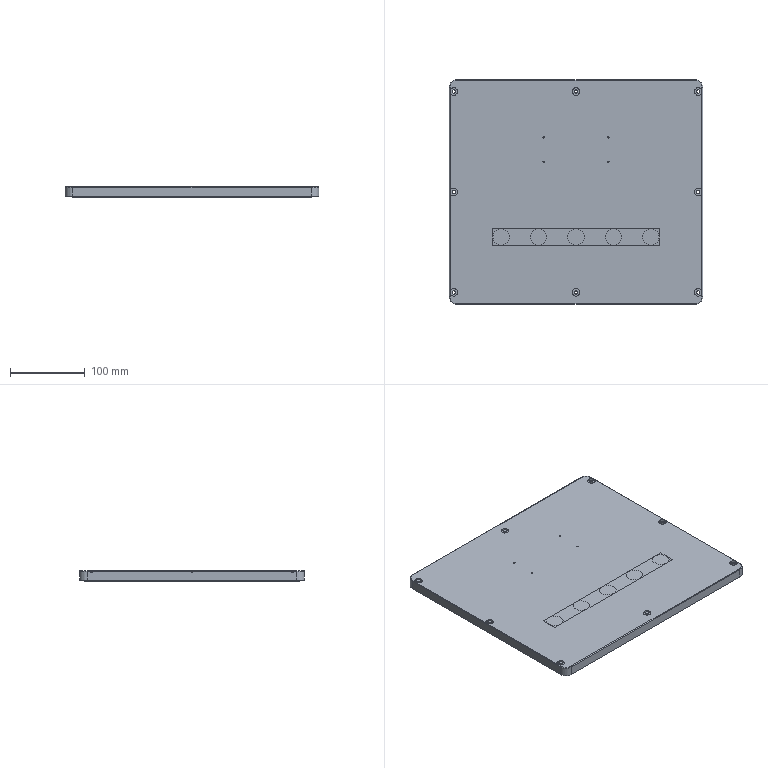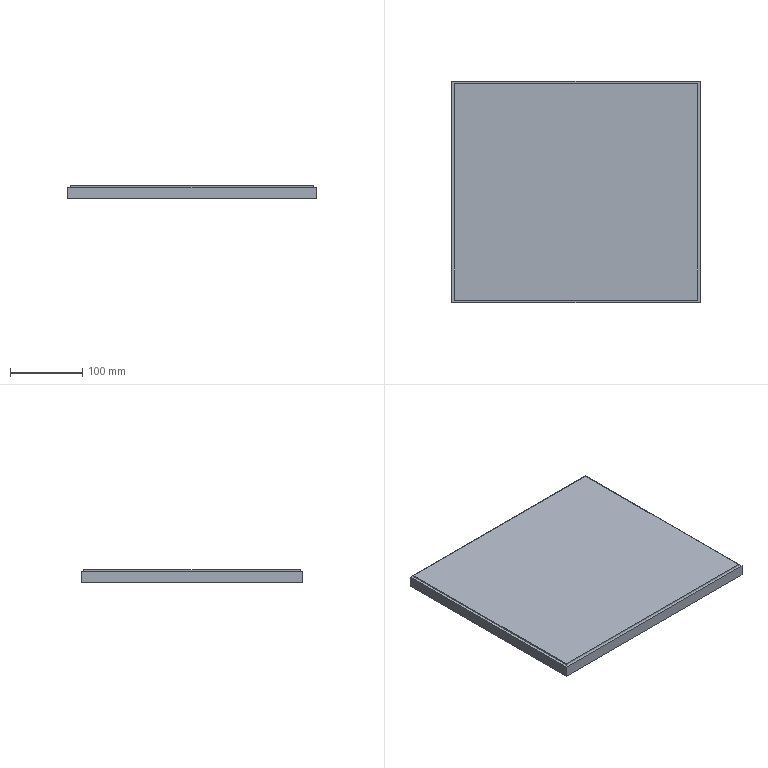CAM job | NX | 3-axis milling, drilling | part box 338 x 300 x 14.5 mm | stock box 345 x 307 x 18 mm
Tools:
number,name,description,diameter,corner_radius,flute_length,length,flutes
3,D63,Milling Tool-5 Parameters,63.0,0.0,50.0,75.0,2
4,D10,Milling Tool-5 Parameters,10.0,0.0,50.0,75.0,2
14,D10JING,Milling Tool-5 Parameters,10.0,0.0,50.0,75.0,2
1,D6A45,Milling Tool-5 Parameters,6.0,0.0,3.0,3.0,2
20,2.1ZT,Drilling Tool,2.05,0.0,35.0,50.0,2
11,4.5ZT,Drilling Tool,4.5,0.0,35.0,50.0,2
7,D3R0.5,Milling Tool-5 Parameters,3.0,0.5,50.0,75.0,2
16,D6,Milling Tool-5 Parameters,6.0,0.0,50.0,75.0,2
22,2.5ZT,Drilling Tool,2.5,0.0,35.0,50.0,2
21,D4A45,Milling Tool-5 Parameters,4.0,0.0,2.0,2.0,2
17,D4,Milling Tool-5 Parameters,4.0,0.0,50.0,75.0,2
Operations:
program,operation,operation_type,tool,method,geometry_group,spindle_rpm,surface_speed,feed_per_tooth,feed_cut,feed_plunge,cut_length_mm,path_length_mm,cut_time_min,machine_time_min
1,FLOOR_WALL,VolumeBased25DMillingOperation,D63,METHOD,A,6500.0,1286.0,0.0962,1250.0,100.0,3149.797,3203.797,2.52,2.525
1,DRILLING_COPY_1,Operation,D6A45,METHOD,A,5000.0,94.0,0.025,250.0,0.0,61.2,1674.06,0.2448,0.4061
1,DRILLING_COPY_COPY,Operation,2.1ZT,METHOD,A,1447.0,10.0,0.0346,100.0,0.0,40.464,302.252,0.4046,0.4308
1,DRILLING_COPY_COPY_COPY,Operation,4.5ZT,METHOD,A,1447.0,10.0,0.0346,100.0,0.0,146.815,1399.848,1.468,1.593
1,ADAPTIVE_MILLING,CavityMilling,D10,METHOD,A,9500.0,298.0,0.1579,3000.0,1000.0,5468.216,6915.074,1.825,1.97
1,HOLE_MILLING,CylinderMilling,D10,METHOD,A,9500.0,0.0,0.0,2200.0,100.0,1175.045,1685.045,0.5341,0.5851
1,ZLEVEL_PROFILE,ZLevelMilling,D10JING,METHOD,A,9500.0,298.0,0.0526,1000.0,100.0,1301.71,1384.71,1.302,1.31
1,ZLEVEL_PROFILE_COPY,ZLevelMilling,D10JING,METHOD,A,9500.0,298.0,0.0526,1000.0,100.0,252.904,1119.534,0.2529,0.3396
1,ZLEVEL_PROFILE_1,ZLevelMilling,D3R0.5,METHOD,A,9500.0,89.0,0.1316,2500.0,1000.0,29109.615,29169.128,11.645,11.651
1,HOLE_MILLING_1,CylinderMilling,D6,METHOD,A,9500.0,179.0,0.0737,1400.0,100.0,653.849,2170.849,0.467,0.6187
1,PLANAR_MILL_COPY_COPY,PlanarMilling,D6A45,METHOD,A,9500.0,179.0,0.0658,1250.0,100.0,605.516,3030.479,0.4844,0.7269
2,FLOOR_WALL_COPY,VolumeBased25DMillingOperation,D63,METHOD,B,6500.0,1286.0,0.0962,1250.0,100.0,12375.187,14053.187,9.9,10.068
2,FLOOR_WALL_COPY_1,VolumeBased25DMillingOperation,D63,METHOD,B,6500.0,1286.0,0.0962,1250.0,100.0,3093.797,3147.797,2.475,2.48
2,CAVITY_MILL_1,CavityMilling,D10,METHOD,B,9500.0,298.0,0.1579,3000.0,1000.0,114634.989,116016.261,38.523,38.661
2,FLOOR_WALL_1,VolumeBased25DMillingOperation,D10,METHOD,B,9500.0,298.0,0.1316,2500.0,1000.0,5125.334,6021.05,2.077,2.167
2,DRILLING_COPY_1_1,Operation,D6A45,METHOD,B,5000.0,94.0,0.025,250.0,0.0,14.4,259.07,0.0576,0.0821
2,DRILLING_COPY_COPY_1,Operation,2.5ZT,METHOD,B,1447.0,10.0,0.0346,100.0,0.0,39.004,308.278,0.39,0.417
2,FLOOR_WALL_1_COPY_1,VolumeBased25DMillingOperation,D10JING,METHOD,B,9500.0,298.0,0.0632,1200.0,1000.0,19205.702,21337.438,16.101,16.339
2,FLOOR_WALL_1_COPY_1_COPY_1,VolumeBased25DMillingOperation,D10JING,METHOD,B,9500.0,298.0,0.0632,1200.0,1000.0,2294.852,2354.852,1.913,1.919
2,HOLE_MILLING_2,CylinderMilling,D4,METHOD,B,9500.0,119.0,0.0711,1350.0,100.0,874.293,2147.293,0.6476,0.7749
2,PLANAR_MILL_COPY_COPY_COPY,PlanarMilling,D6A45,METHOD,B,9500.0,179.0,0.0658,1250.0,100.0,375.579,1736.101,0.3005,0.4365
2,PLANAR_MILL_COPY_COPY_COPY_COPY,PlanarMilling,D6A45,METHOD,B,9500.0,179.0,0.0658,1250.0,100.0,491.738,1001.692,0.3934,0.4444
2,PLANAR_MILL_COPY_COPY_COPY_COPY_COPY,PlanarMilling,D6A45,METHOD,B,9500.0,179.0,0.0658,1250.0,100.0,2371.729,2496.028,1.897,1.91
2,ZLEVEL_PROFILE_2_COPY,ZLevelMilling,D4A45,METHOD,B,9500.0,179.0,0.0658,1250.0,100.0,2534.003,4653.163,2.027,2.239
2,刀补14,VolumeBased25DMillingOperation,D10JING,METHOD,B,9500.0,298.0,0.0632,1200.0,1000.0,2378.495,2789.122,1.983,2.024
UNUSED,ADAPTIVE_MILLING_COPY,CavityMilling,D10,METHOD,B,9500.0,298.0,0.1579,3000.0,1000.0,106677.911,108733.866,36.058,36.264